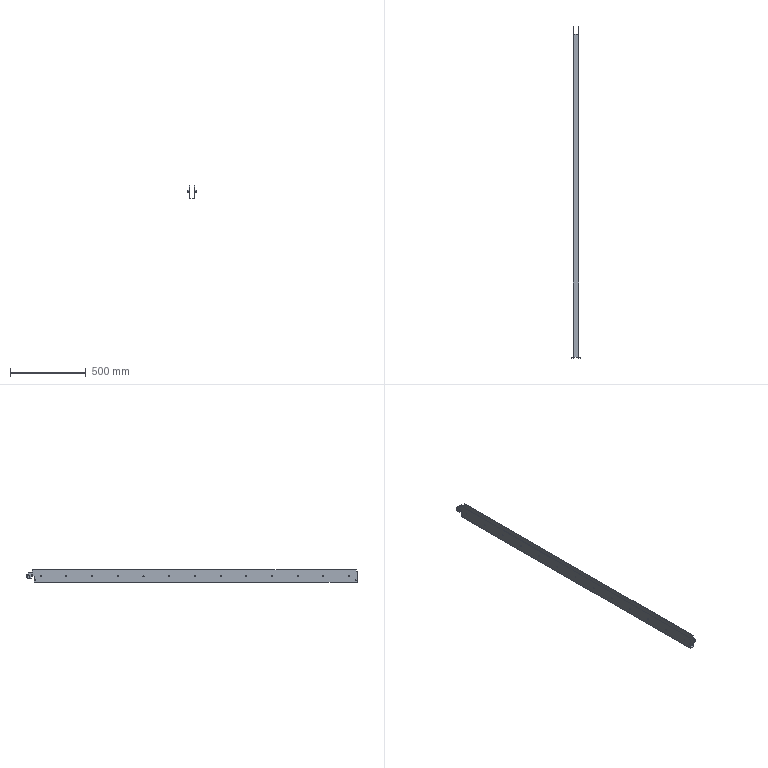Part | NX | features solid 2 | 1 solid | 222 faces | box 62 x 2196 x 85 mm | volume 647771 mm3 | plane 86 | cylinder 82 | cone 54 | commonest cylinder face diameters 7.14 x26 6 x20 2 x14 3.4 x12 6.5 x4 1.5 x2